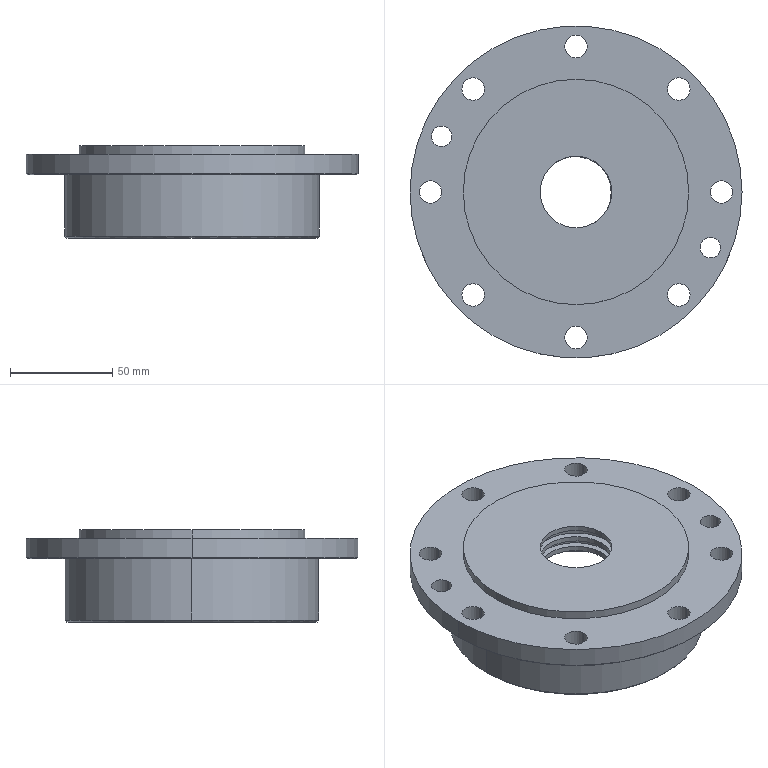Part | SolidWorks | features ICE 12, Chamfer 2, HoleWzd 2, CirPattern 1, Extrusion 1 | 1 solid | 63 faces | box 162 x 162 x 45 mm | volume 267421 mm3 | cylinder 46 | plane 13 | cone 4 | commonest cylinder face diameters 11 x16 35 x6 10 x4 40.6 x4 100 x2 110 x2